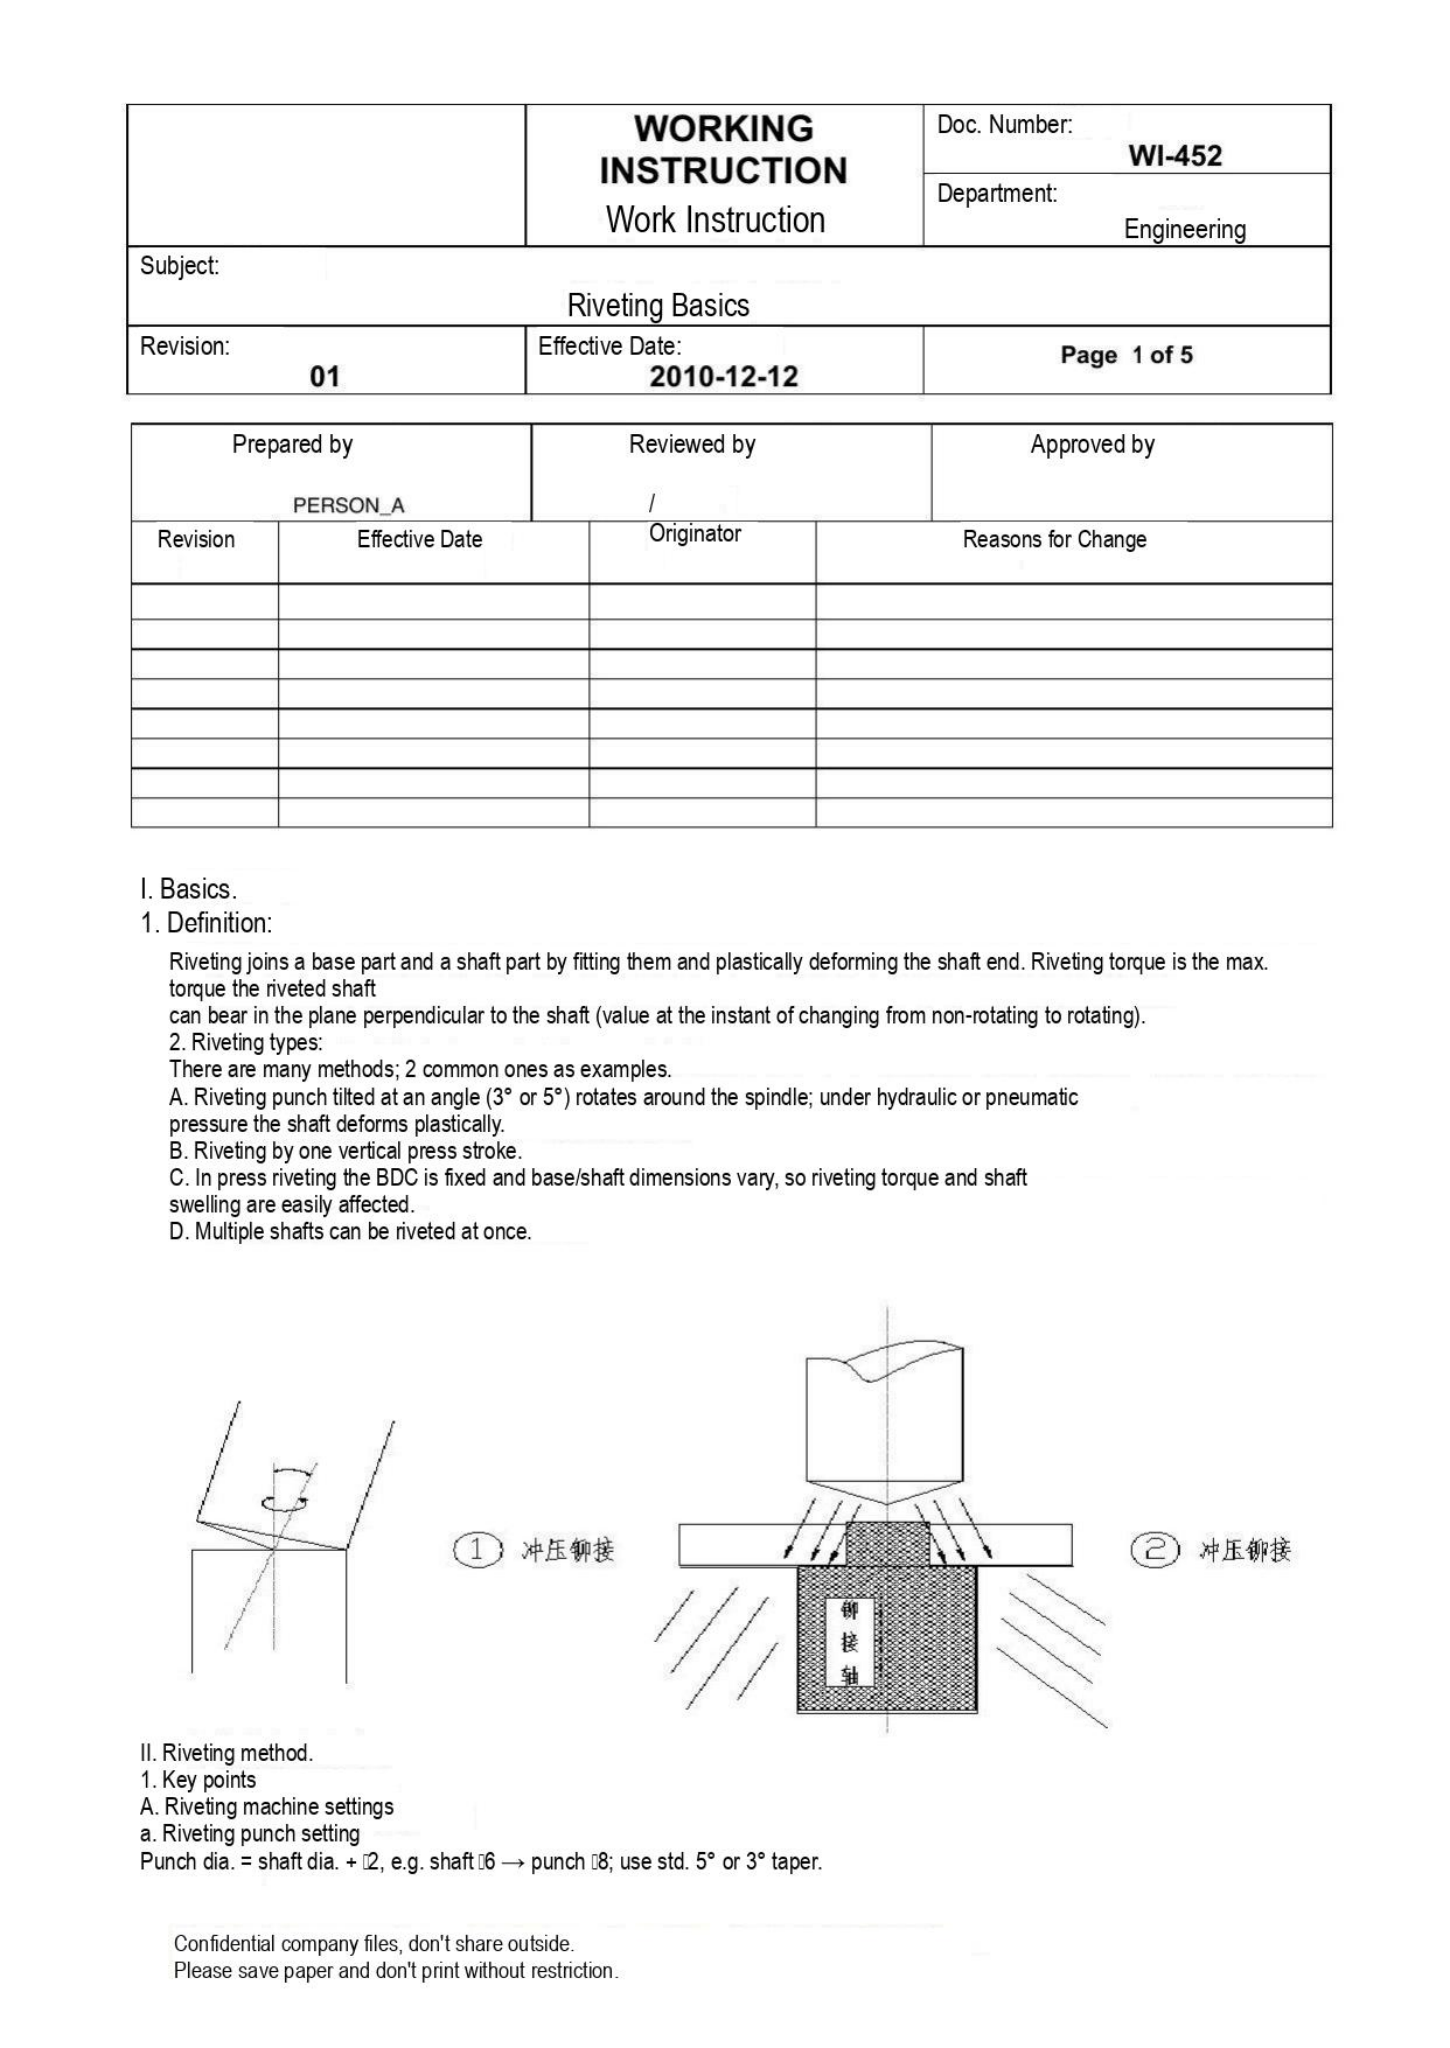| | WORKING INSTRUCTION<br>Work Instruction | Doc. Number: WI-452<br>Department: Engineering |
|---|---|---|
| Subject: Riveting Basics | | |
| Revision: 01 | Effective Date: 2010-12-12 | Page 1 of 5 |

| Prepared by | Reviewed by | Approved by |
|---|---|---|
| PERSON_A | / | |

| Revision | Effective Date | Originator | Reasons for Change |
|---|---|---|---|
| | | | |
| | | | |
| | | | |
| | | | |
| | | | |
| | | | |
| | | | |
| | | | |

I. Basics.
1. Definition:
Riveting joins a base part and a shaft part by fitting them and plastically deforming the shaft end. Riveting torque is the max. torque the riveted shaft
can bear in the plane perpendicular to the shaft (value at the instant of changing from non-rotating to rotating).
2. Riveting types:
There are many methods; 2 common ones as examples.
A. Riveting punch tilted at an angle (3° or 5°) rotates around the spindle; under hydraulic or pneumatic pressure the shaft deforms plastically.
B. Riveting by one vertical press stroke.
C. In press riveting the BDC is fixed and base/shaft dimensions vary, so riveting torque and shaft swelling are easily affected.
D. Multiple shafts can be riveted at once.

① 冲压铆接

铆接轴

② 冲压铆接

II. Riveting method.
1. Key points
A. Riveting machine settings
a. Riveting punch setting
Punch dia. = shaft dia. + □2, e.g. shaft □6 → punch □8; use std. 5° or 3° taper.

Confidential company files, don't share outside.
Please save paper and don't print without restriction.
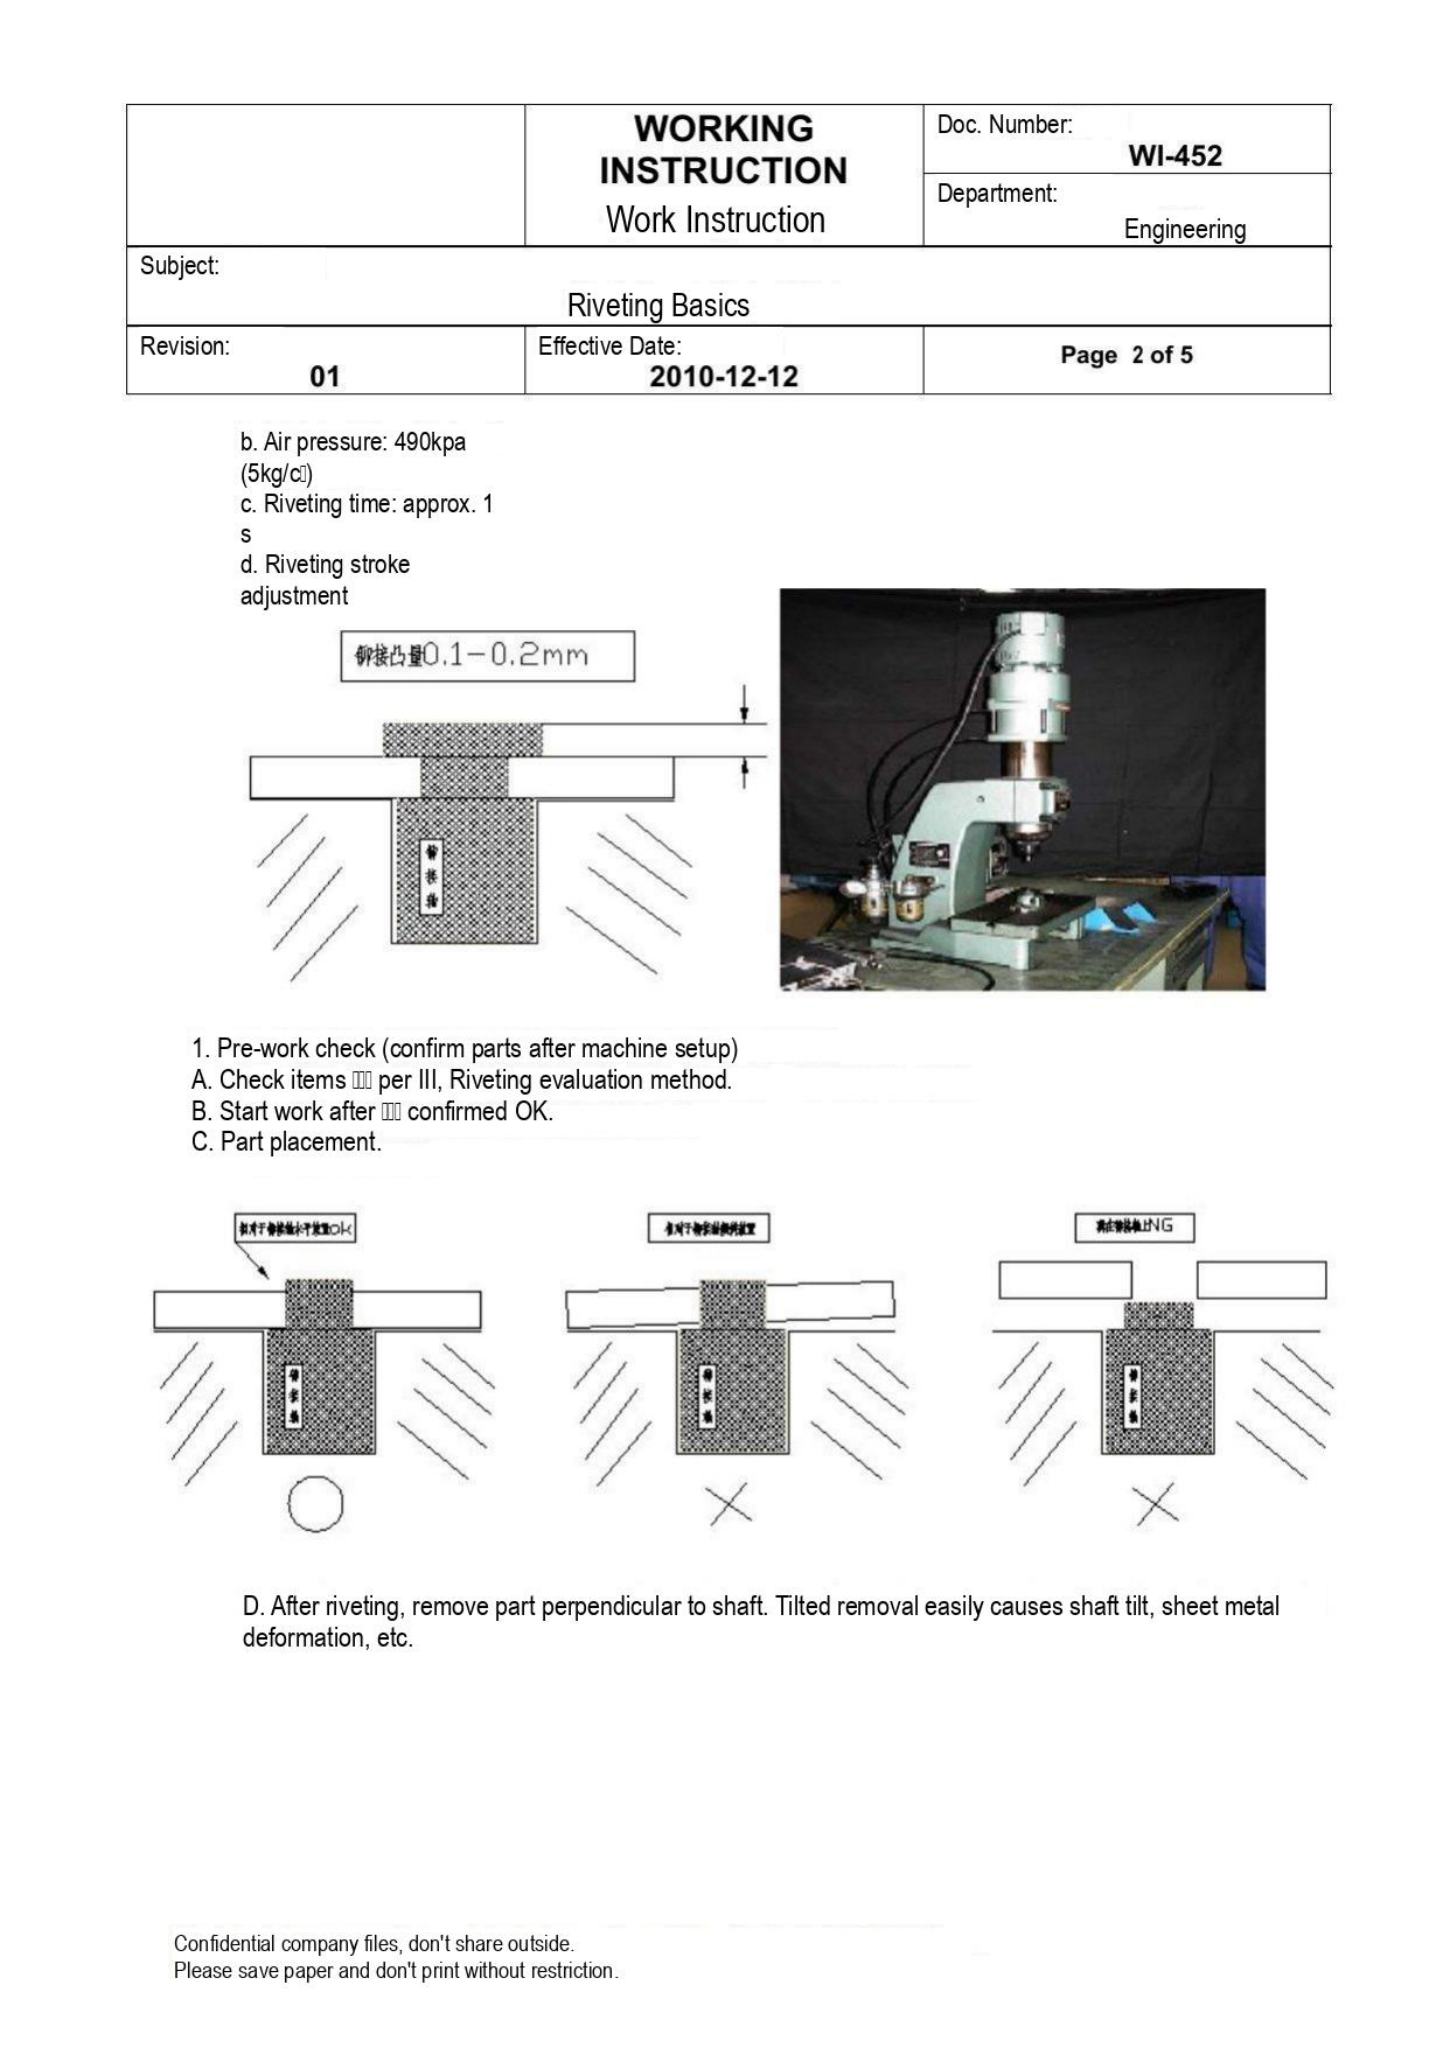| | WORKING INSTRUCTION<br>Work Instruction | Doc. Number: WI-452<br>Department: Engineering |
|---|---|---|
| Subject: Riveting Basics | | |
| Revision: 01 | Effective Date: 2010-12-12 | Page 2 of 5 |

b. Air pressure: 490kpa (5kg/c)
c. Riveting time: approx. 1 s
d. Riveting stroke adjustment

铆接凸量0.1-0.2mm

1. Pre-work check (confirm parts after machine setup)
A. Check items per III, Riveting evaluation method.
B. Start work after confirmed OK.
C. Part placement.

OK

NG

D. After riveting, remove part perpendicular to shaft. Tilted removal easily causes shaft tilt, sheet metal deformation, etc.

Confidential company files, don't share outside.
Please save paper and don't print without restriction.
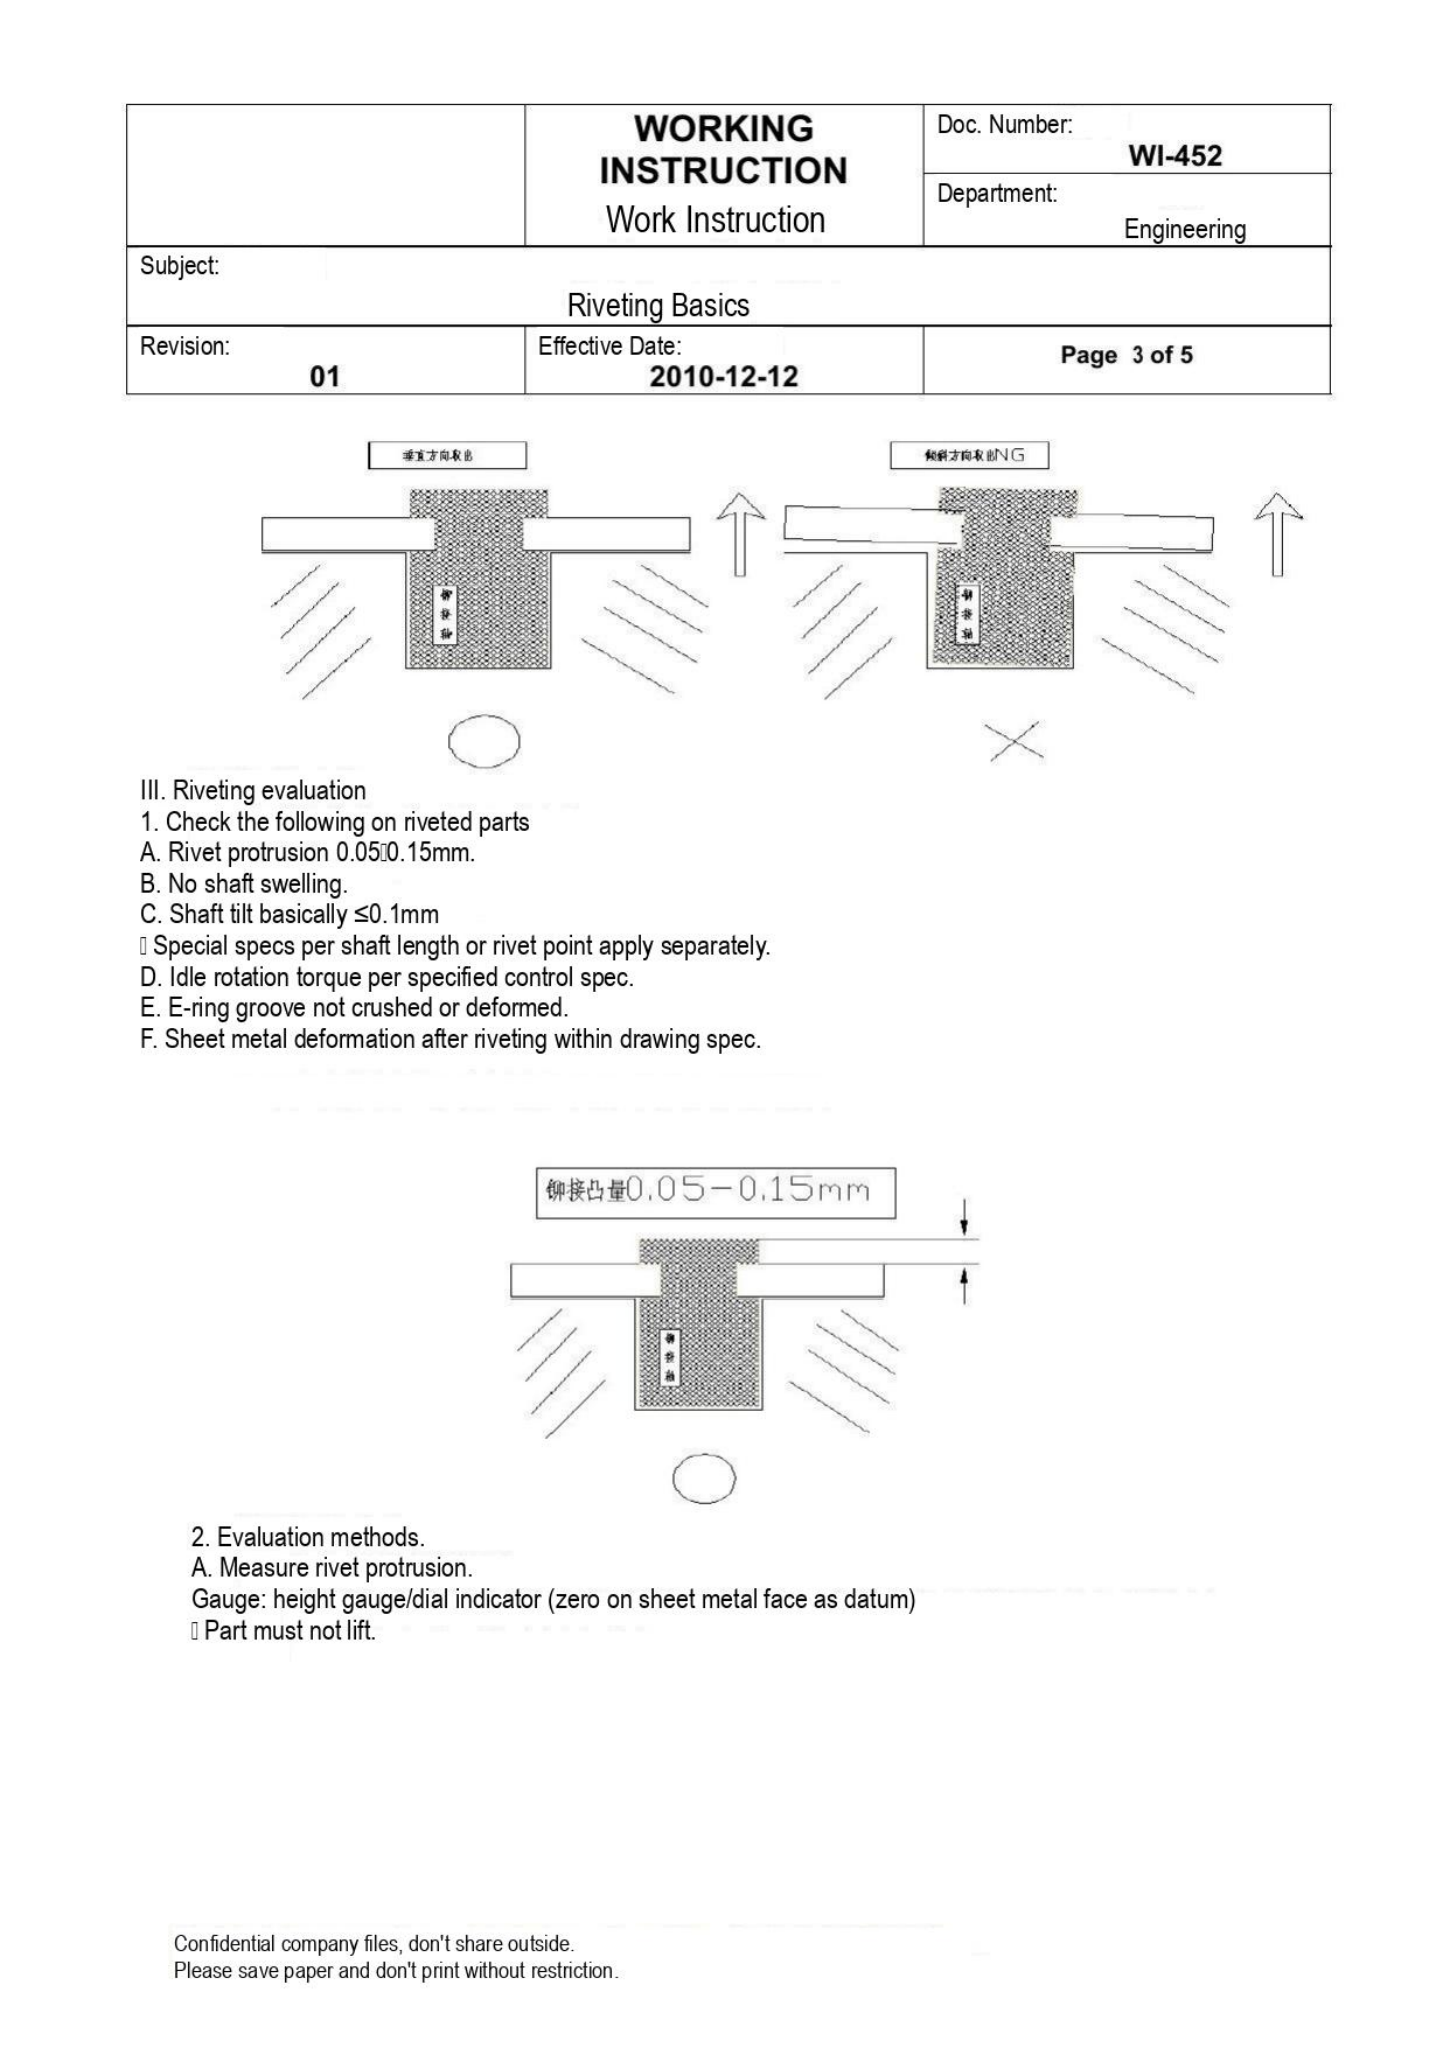| | WORKING INSTRUCTION<br>Work Instruction | Doc. Number: WI-452<br>Department: Engineering |
|---|---|---|
| Subject: Riveting Basics | | |
| Revision: 01 | Effective Date: 2010-12-12 | Page 3 of 5 |

垂直方向取出

铆接轴

倾斜方向取出NG

铆接轴

III. Riveting evaluation
1. Check the following on riveted parts
A. Rivet protrusion 0.050.15mm.
B. No shaft swelling.
C. Shaft tilt basically ≤0.1mm
 Special specs per shaft length or rivet point apply separately.
D. Idle rotation torque per specified control spec.
E. E-ring groove not crushed or deformed.
F. Sheet metal deformation after riveting within drawing spec.

铆接凸量0.05−0.15mm

铆接轴

2. Evaluation methods.
A. Measure rivet protrusion.
Gauge: height gauge/dial indicator (zero on sheet metal face as datum)
 Part must not lift.

Confidential company files, don't share outside.
Please save paper and don't print without restriction.
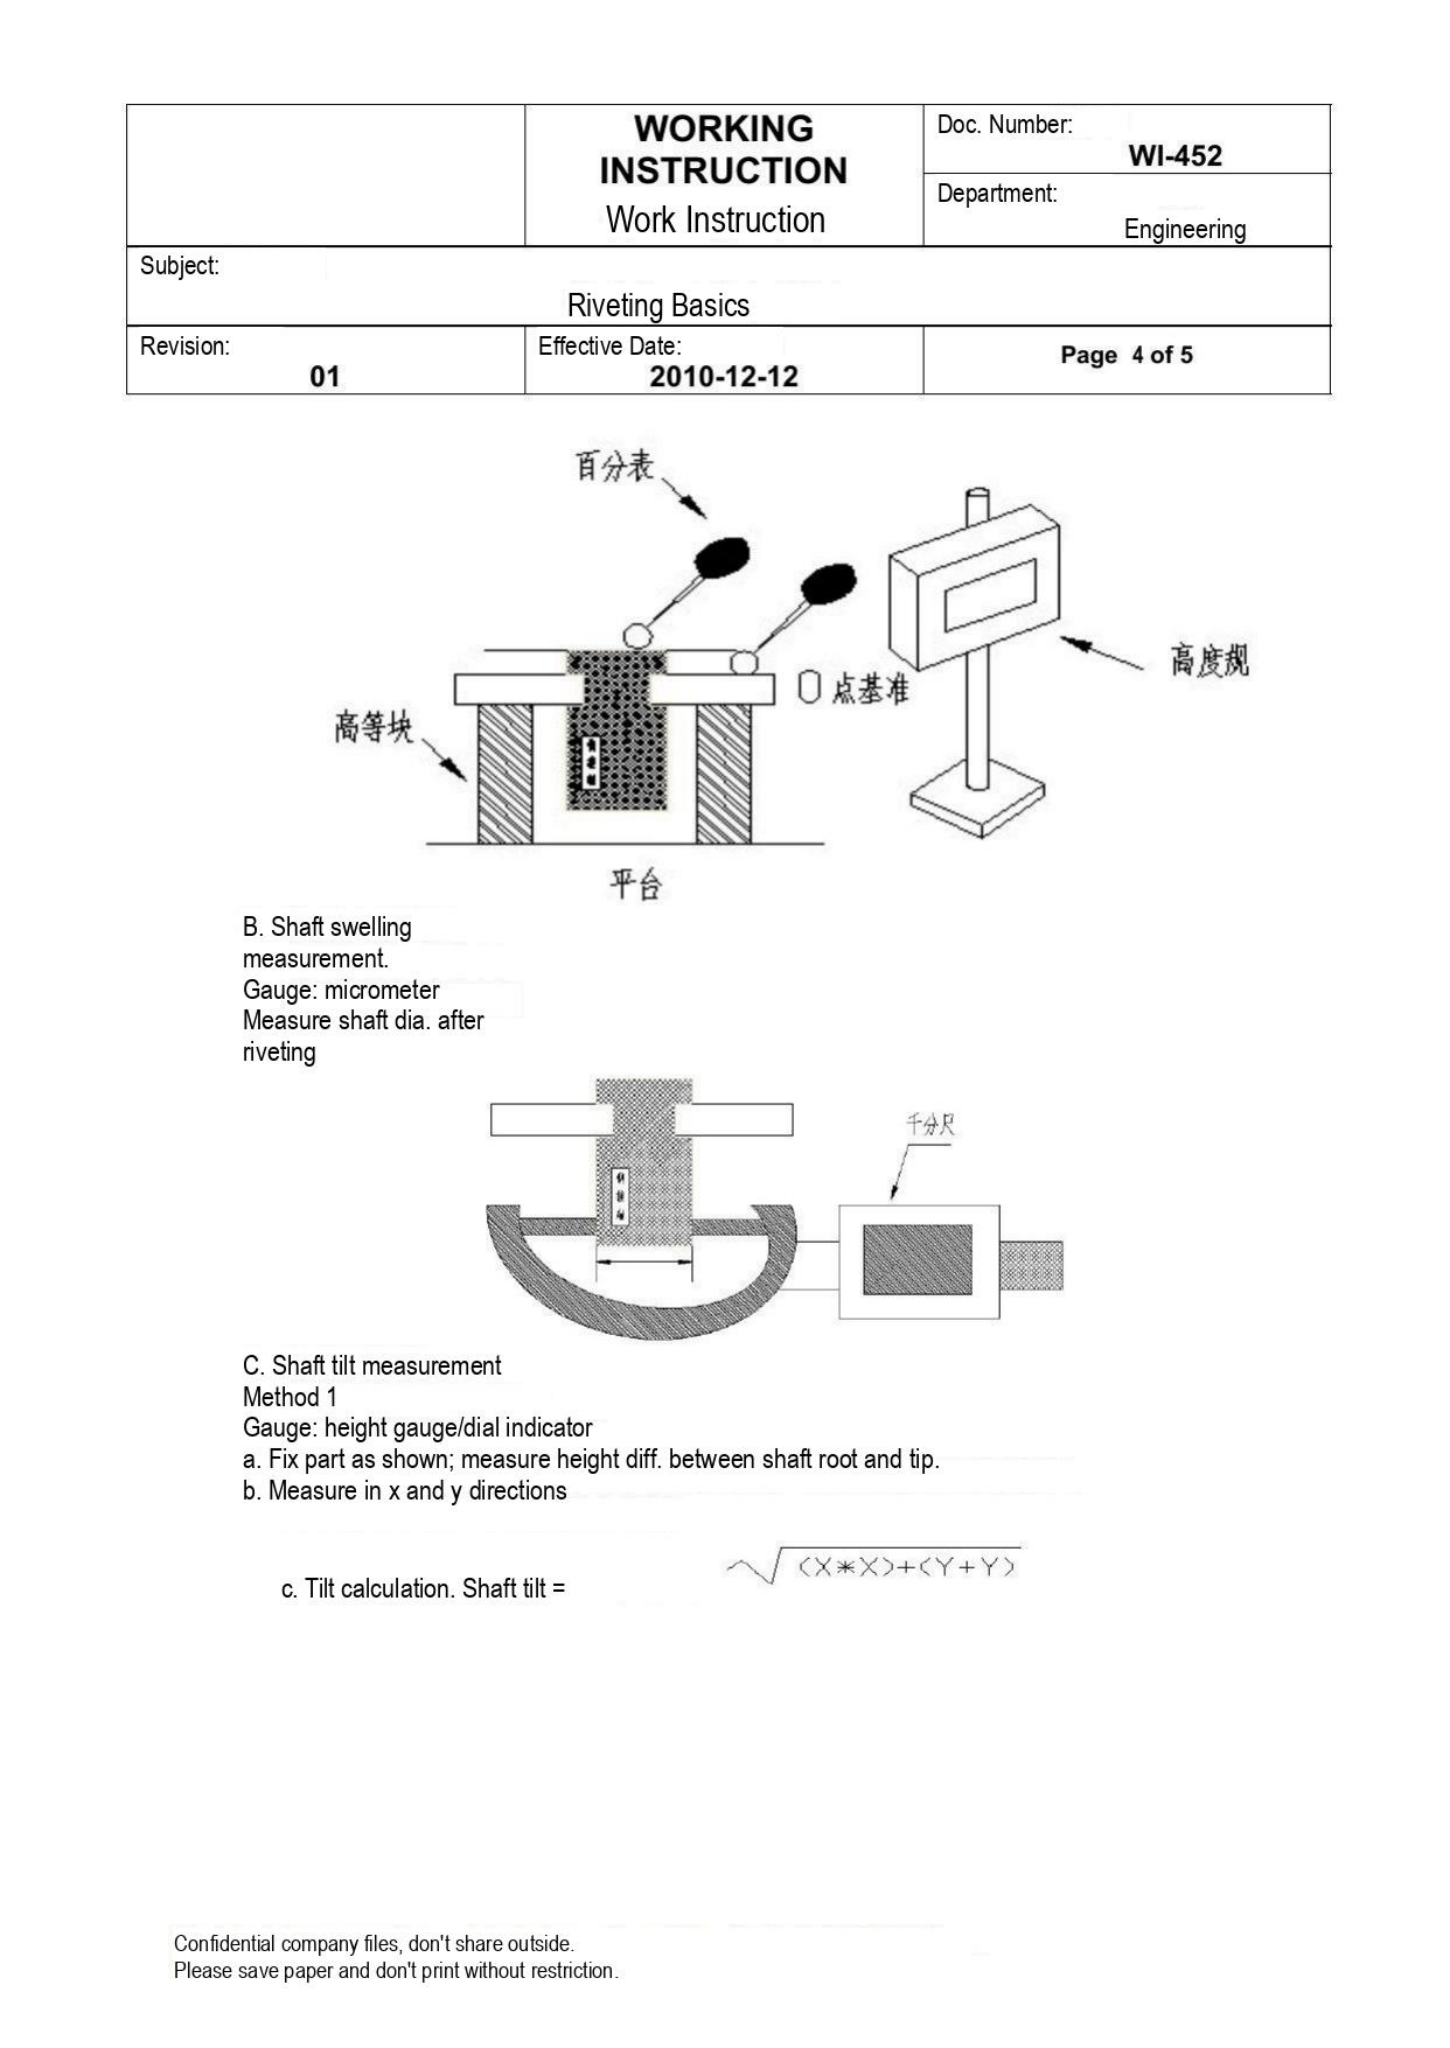| | WORKING INSTRUCTION<br>Work Instruction | Doc. Number: WI-452<br>Department: Engineering |
|---|---|---|
| Subject: Riveting Basics | | |
| Revision: 01 | Effective Date: 2010-12-12 | Page 4 of 5 |

百分表

高度规

0点基准

高等块

平台

B. Shaft swelling measurement.
Gauge: micrometer
Measure shaft dia. after riveting

千分尺

C. Shaft tilt measurement
Method 1
Gauge: height gauge/dial indicator
a. Fix part as shown; measure height diff. between shaft root and tip.
b. Measure in x and y directions

c. Tilt calculation. Shaft tilt = √ (X*X)+(Y+Y)

Confidential company files, don't share outside.
Please save paper and don't print without restriction.
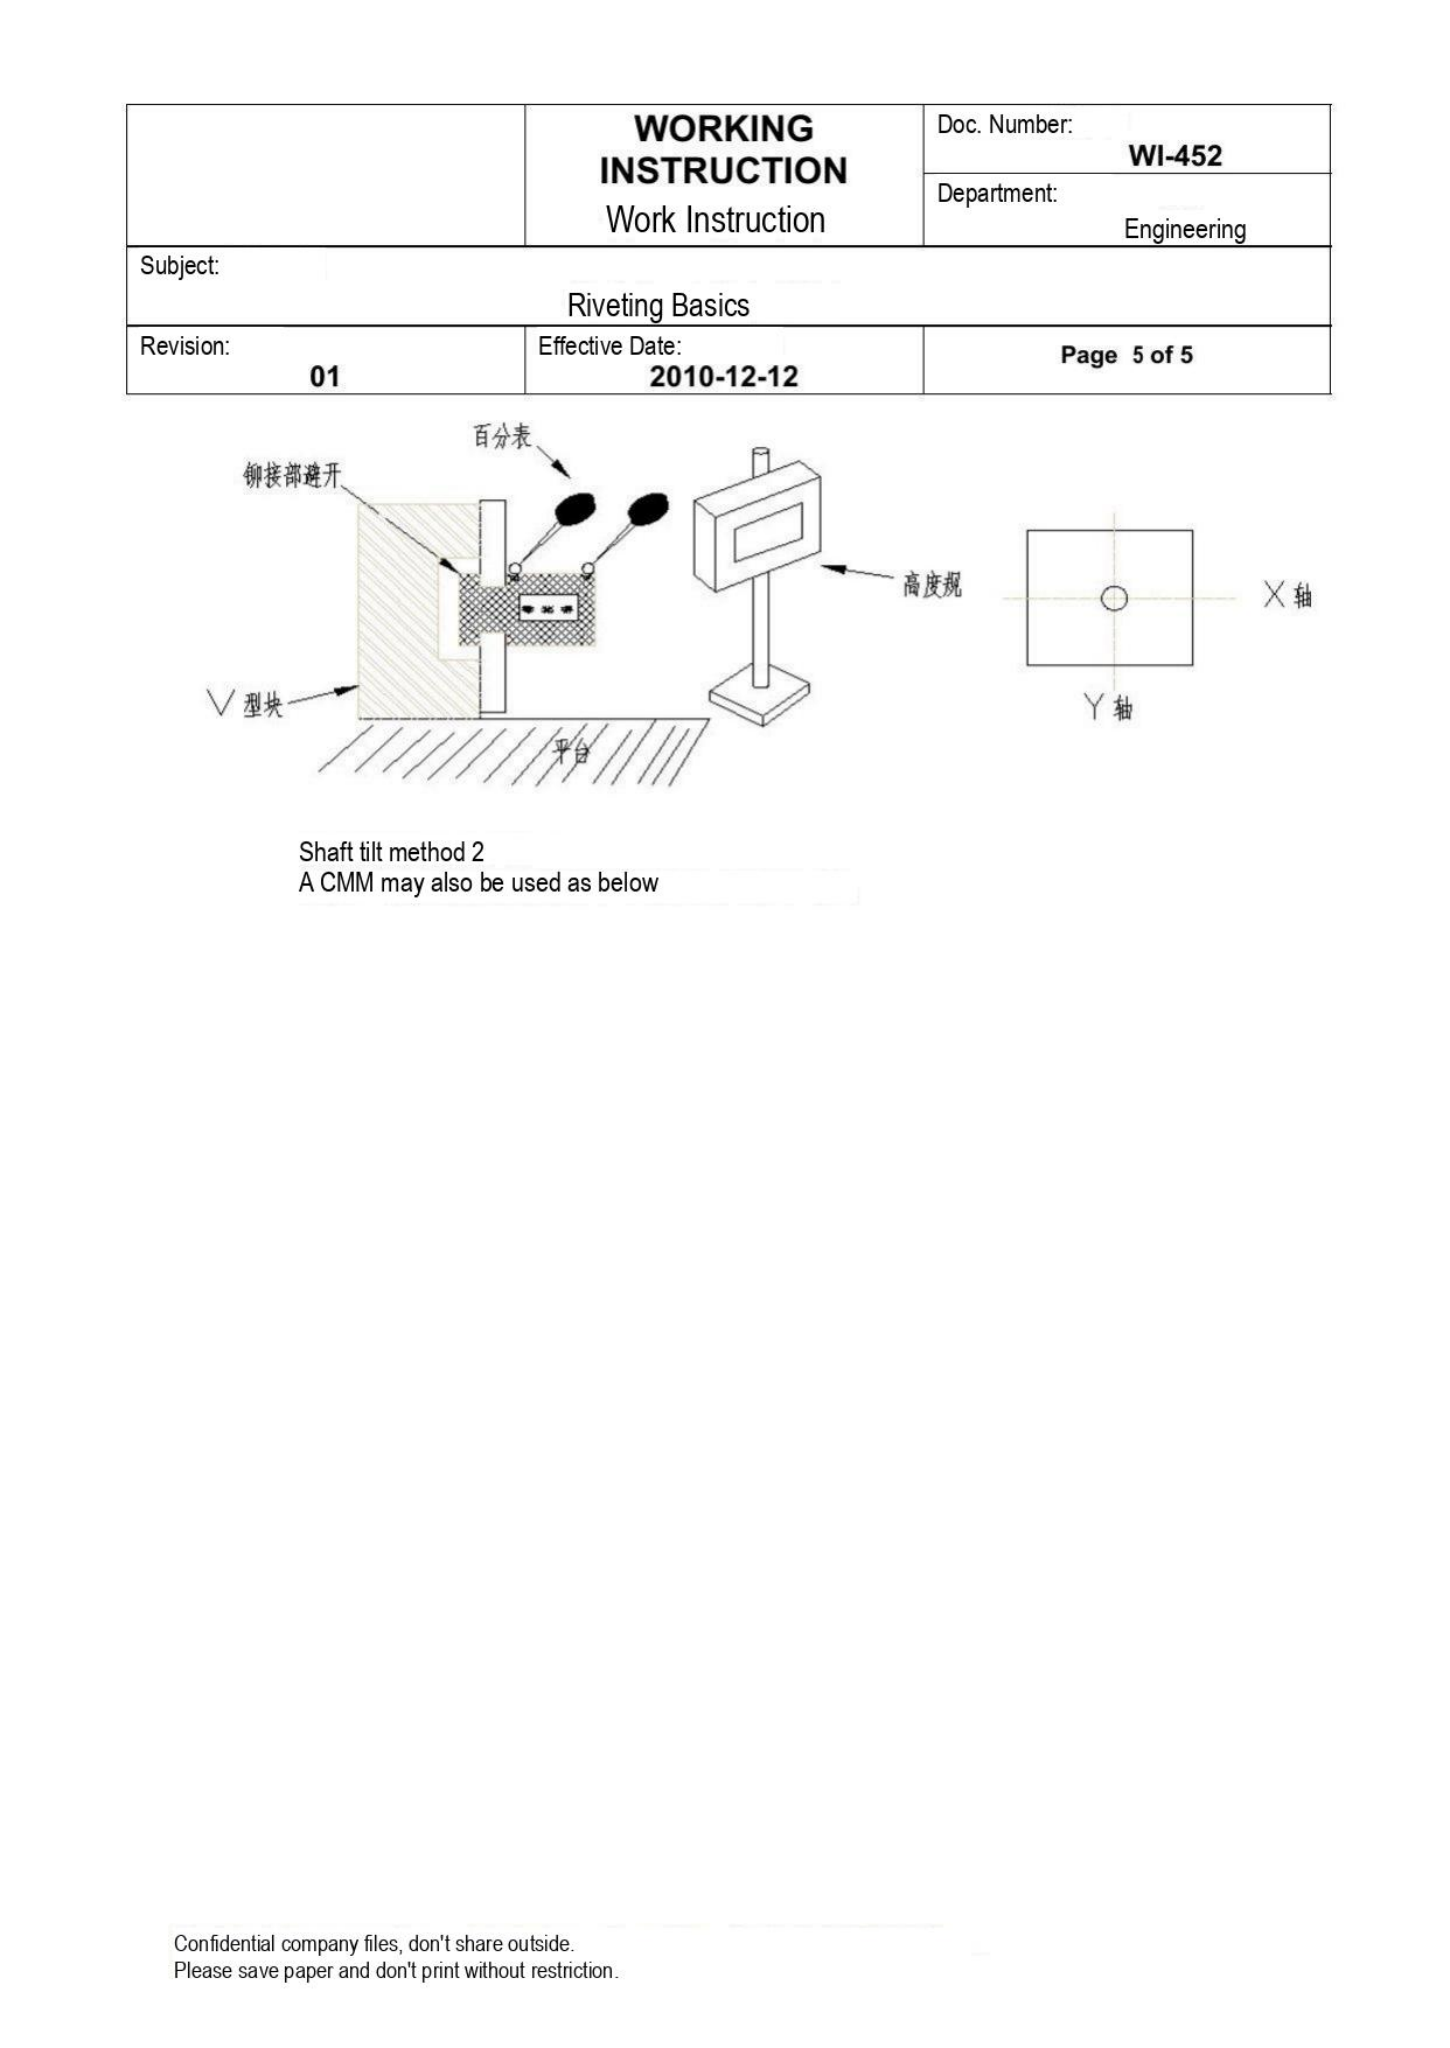| | WORKING INSTRUCTION<br>Work Instruction | Doc. Number:<br>WI-452<br><br>Department:<br>Engineering |
|---|---|---|
| Subject:<br>Riveting Basics | | |
| Revision:<br>01 | Effective Date:<br>2010-12-12 | Page 5 of 5 |

百分表

铆接部避开

高度规

X 轴

V 型块

Y 轴

平台

Shaft tilt method 2
A CMM may also be used as below

Confidential company files, don't share outside.
Please save paper and don't print without restriction.